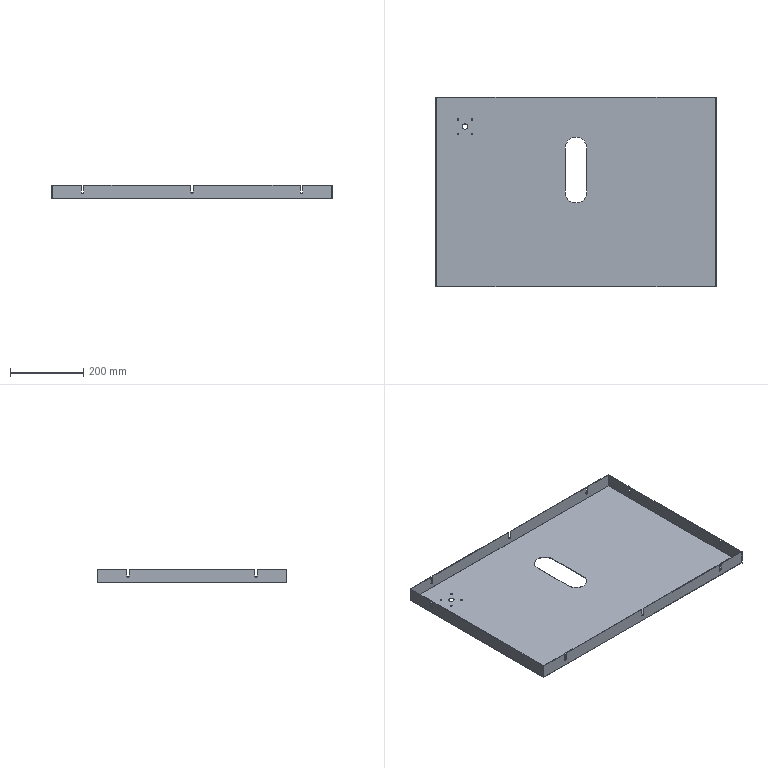Part | STEP file | Top seal plate | 1 solid | 68 faces | box 768 x 518 x 38 mm | volume 719559 mm3 | plane 42 | cylinder 26 | commonest cylinder face diameters 7 x14 4 x8 15 x2 60 x2